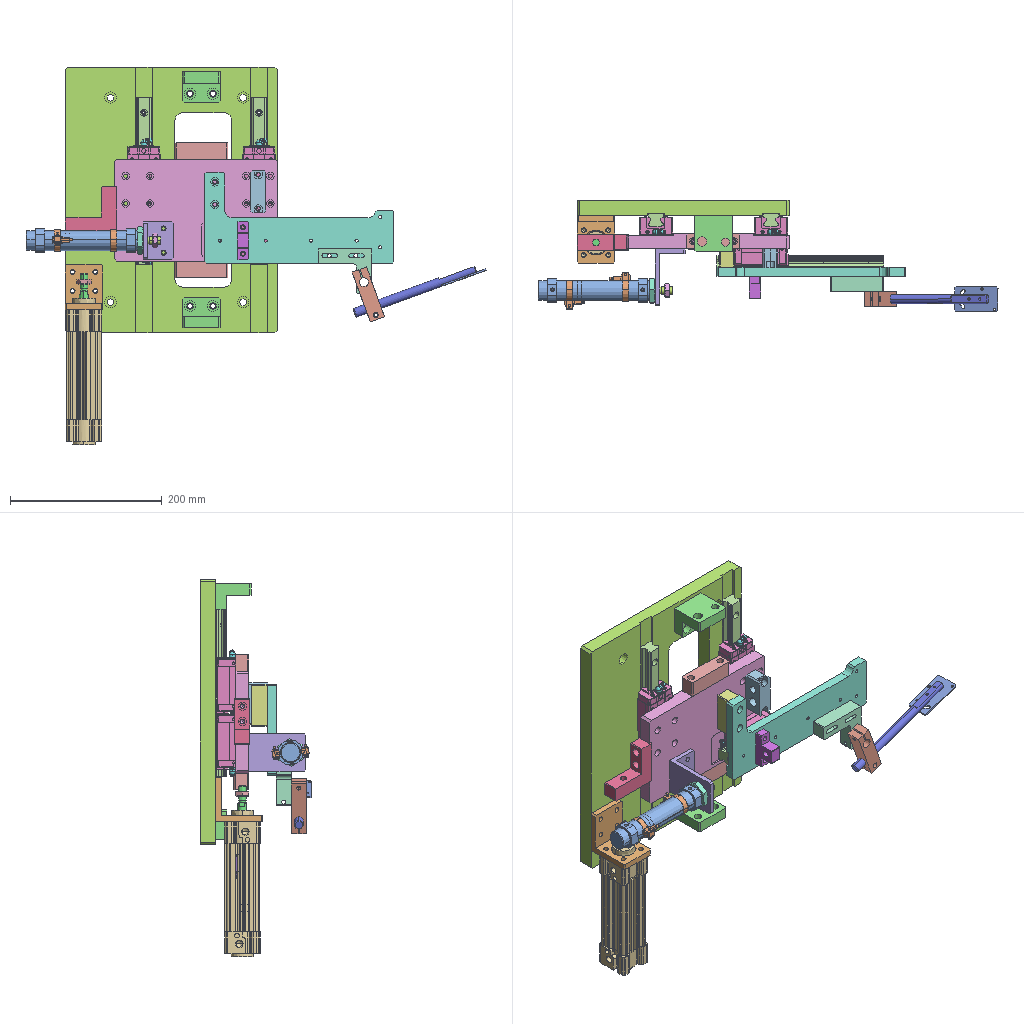Assembly | SolidWorks | 31 different items | 46 placed | box 607 x 147 x 498 mm
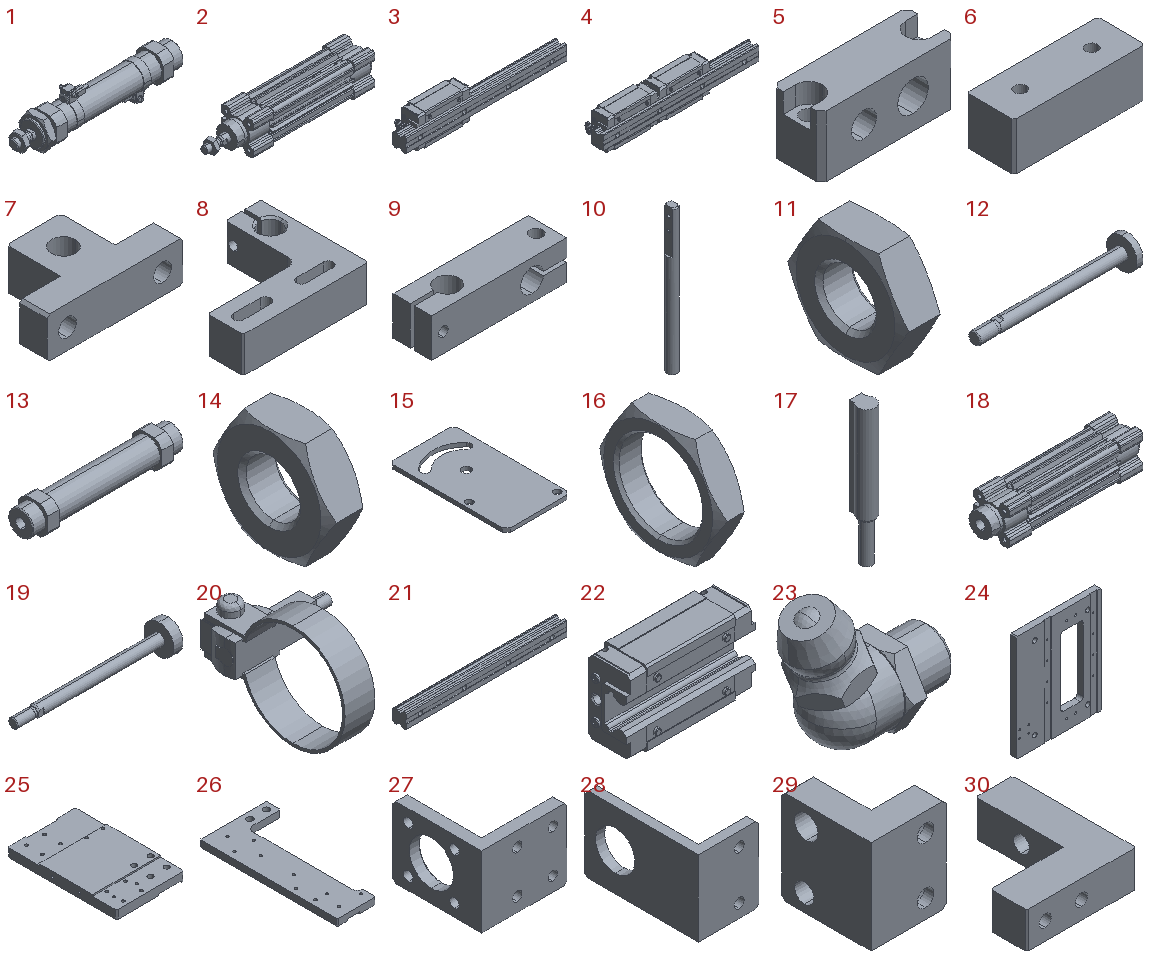Parts list (item | name | quantity | parent item | size | volume | features):
1 | (subassembly) | x1 | - | 178 x 36.95 x 48.66 mm | 71488 mm3 | -
2 | (subassembly) | x1 | - | 226 x 47 x 47 mm | 241103 mm3 | -
3 | (subassembly) | x1 | - | 220 x 30 x 44 mm | 122674 mm3 | -
4 | (subassembly) | x2 | - | 220.441 x 30 x 44 mm | 182432 mm3 | -
5 | - | x1 | - | 55 x 20 x 25 mm | 20408 mm3 | features HoleWzd 3, Chamfer 1, Extrusion 1, ICE 1
6 | - | x1 | - | 55 x 20 x 20 mm | 21175 mm3 | features Chamfer 1, Extrusion 1, HoleWzd 1
7 | - | x1 | - | 50 x 30 x 15 mm | 11868 mm3 | features HoleWzd 2, Chamfer 1, Extrusion 1
8 | - | x1 | - | 70 x 60 x 20 mm | 36605 mm3 | features Chamfer 2, HoleWzd 2, Extrusion 1, Fillet 1
9 | - | x1 | - | 70 x 20 x 20 mm | 21545 mm3 | features HoleWzd 4, Extrusion 1, ICE 1
10 | - | x1 | - | 12 x 12 x 170 mm | 17822 mm3 | features Chamfer 1, Extrusion 1, HoleWzd 1, ICE 1
11 | - | x1 | in 2 | 6 x 19.63 x 17 mm | 1121 mm3 | features BaseBody 1
12 | - | x1 | in 1 | 126 x 25 x 25 mm | 11883 mm3 | features BaseBody 1
13 | - | x1 | in 1 | 157 x 30 x 30 mm | 51247 mm3 | features BaseBody 1
14 | - | x1 | in 1 | 6 x 19.63 x 17 mm | 1117 mm3 | features BaseBody 1
15 | - | x1 | - | 33 x 60 x 2 mm | 3630 mm3 | features Chamfer 1, Extrusion 1
16 | - | x1 | in 1 | 8 x 36.95 x 32 mm | 3211 mm3 | features BaseBody 1
17 | - | x2 | in 2 | 4 x 4.6 x 32 mm | 381.799 mm3 | features BaseBody 1
18 | - | x1 | in 2 | 193 x 47 x 47 mm | 214330 mm3 | features BaseBody 1
19 | - | x1 | in 2 | 166.9 x 32 x 32 mm | 24888 mm3 | features BaseBody 1
20 | - | x2 | in 1 | 27.005 x 38.33 x 28 mm | 2014 mm3 | features BaseBody 1
21 | - | x3 | in 3, 4 | 220 x 18 x 20 mm | 62917 mm3 | features BaseBody 1
22 | - | x5 | in 3, 4 | 74 x 26 x 44 mm | 58956 mm3 | features BaseBody 1
23 | - | x5 | in 3, 4 | 16.6 x 9.238 x 15.311 mm | 801.451 mm3 | features BaseBody 1
24 | - | x1 | - | 280 x 20 x 350 mm | 1546665 mm3 | features HoleWzd 6, Chamfer 1, Extrusion 1, Fillet 1, ICE 1
25 | - | x1 | - | 134 x 215 x 20 mm | 503550 mm3 | features HoleWzd 8, ICE 2, Chamfer 1, Extrusion 1
26 | - | x1 | - | 120 x 249 x 12 mm | 181549 mm3 | features HoleWzd 5, Chamfer 1, Extrusion 1, ICE 1
27 | - | x1 | - | 60 x 62.5 x 50 mm | 37459 mm3 | features HoleWzd 3, Chamfer 2, Extrusion 1
28 | - | x1 | - | 40 x 75 x 50 mm | 29056 mm3 | features HoleWzd 2, Chamfer 1, Extrusion 1
29 | - | x2 | - | 40 x 47.5 x 50 mm | 47018 mm3 | features HoleWzd 3, Chamfer 1, Extrusion 1
30 | - | x1 | - | 60 x 68 x 20 mm | 39349 mm3 | features HoleWzd 2, Chamfer 1, Extrusion 1
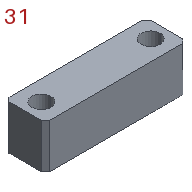31 | - | x2 | - | 70 x 20 x 22 mm | 28656 mm3 | features Chamfer 1, Extrusion 1, HoleWzd 1
Mates (type | each side: item.copy, entity, surface, feature):
In the top assembly
Concentric | 24.1 face cylinder M4 Tapped Hole1 | 21.1 face cylinder Input1 | 2 times
Coincident | 24.1 face plane Boss-Extrude1 | 21.1 face plane Input1
Concentric | 24.1 face cylinder M4 Tapped Hole1 | 21.2 face cylinder Input1 | 2 times
Coincident | 24.1 face plane Boss-Extrude1 | 21.2 face plane Input1
Concentric | 25.1 face cylinder M6 Tapped Hole1 | 30.1 face cylinder Hole1 | 2 times
Coincident | 25.1 face plane Cut-Extrude1 | 30.1 face plane Boss-Extrude1
Coincident | 25.1 face plane Boss-Extrude1 | 22.1 face plane Input1
Width | 25.1 face plane Boss-Extrude1 | 25.1 face plane Boss-Extrude1 | 22.2 face plane Input1 | 22.1 face plane Input1
Concentric | 31.1 face cylinder Hole1 | 25.1 face cylinder M5 Tapped Hole2 | 2 times
Coincident | 31.1 face plane Boss-Extrude1 | 25.1 face plane Boss-Extrude1
Concentric | 25.1 face cylinder M5 Tapped Hole1 | 31.2 face cylinder Hole1 | 2 times
Coincident | 25.1 face plane Boss-Extrude1 | 31.2 face plane Boss-Extrude1
Concentric | 25.1 face cylinder Hole2 | 22.3 face cylinder Input1 | 2 times
Coincident | 25.1 face plane Cut-Extrude2 | 22.3 face plane Input1
Concentric | 26.1 face cylinder M5 Tapped Hole1 | 21.3 face cylinder Input1 | 2 times
Coincident | 26.1 face plane Cut-Extrude1 | 21.3 face plane Input1
Concentric | 24.1 face cylinder M6 Tapped Hole2 | 27.1 face cylinder Hole3 | 2 times
Coincident | 24.1 face plane Boss-Extrude1 | 27.1 face plane Boss-Extrude1
Concentric | 27.1 face cylinder Hole2 | 18.1 face cone Input1
Concentric | 27.1 face cylinder Hole1 | 18.1 face cylinder Input1
Coincident | 27.1 face plane Boss-Extrude1 | 18.1 face plane Input1
Concentric | 25.1 face cylinder M6 Tapped Hole2 | 28.1 face cylinder Hole4 | 2 times
Coincident | 25.1 face plane Boss-Extrude1 | 28.1 face plane Boss-Extrude1
Concentric | 28.1 face cylinder Hole2 | 13.1 face cylinder Input1
Coincident | 28.1 face plane Boss-Extrude1 | 16.1 face plane Input1
Concentric | 24.1 face cylinder M8 Tapped Hole1 | 29.1 face cylinder Hole4 | 2 times
Coincident | 24.1 face plane Boss-Extrude1 | 29.1 face plane Boss-Extrude1
Concentric | 24.1 face cylinder M8 Tapped Hole1 | 29.2 face cylinder Hole4 | 2 times
Coincident | 24.1 face plane Boss-Extrude1 | 29.2 face plane Boss-Extrude1
Concentric | 26.1 face cylinder M5 Tapped Hole3 | 7.1 face cylinder Hole1 | 2 times
Coincident | 26.1 face plane Boss-Extrude1 | 7.1 face plane Boss-Extrude1
Concentric | 25.1 face cylinder M6 Tapped Hole3 | 5.1 face cylinder Hole1 | 2 times
Coincident | 25.1 face plane Boss-Extrude1 | 5.1 face plane Boss-Extrude1
Coincident | 26.1 face plane Boss-Extrude1 | 8.1 face plane Boss-Extrude1 | 2 times
Concentric | 8.1 face cylinder Boss-Extrude1 | 9.1 face cylinder Cut-Extrude1
Coincident | 8.1 face plane Boss-Extrude1 | 9.1 face plane Boss-Extrude1
Lock | 26.1 select_type:0 | 8.1 select_type:0
Concentric | 9.1 face cylinder Boss-Extrude1 | 10.1 face cylinder Boss-Extrude1
Concentric | 15.1 face cylinder Boss-Extrude1 | 10.1 face cylinder M4 Tapped Hole1
Coincident | 15.1 face plane Boss-Extrude1 | 10.1 face plane Cut-Extrude1
Concentric | 26.1 face cylinder Hole1 | 6.1 face cylinder M6 Tapped Hole1 | 2 times
Coincident | 26.1 face plane Boss-Extrude1 | 6.1 face plane Boss-Extrude1
In subassembly 3
DistanceDim | 22.4 face plane Input1 | 21.4 face plane Input1 | 2 times
Lock | 22.4 select_type:0 | 23.1 select_type:0
In subassembly 4
DistanceDim | 22.4 face plane Input1 | 21.4 face plane Input1 | 2 times
DistanceDim | 22.5 face plane Input1 | 21.4 face plane Input1 | 2 times
Lock | 22.4 select_type:0 | 23.1 select_type:0
Lock | 22.5 select_type:0 | 23.2 select_type:0
Coincident | 22.4 face plane Input1 | 22.5 face plane Input1